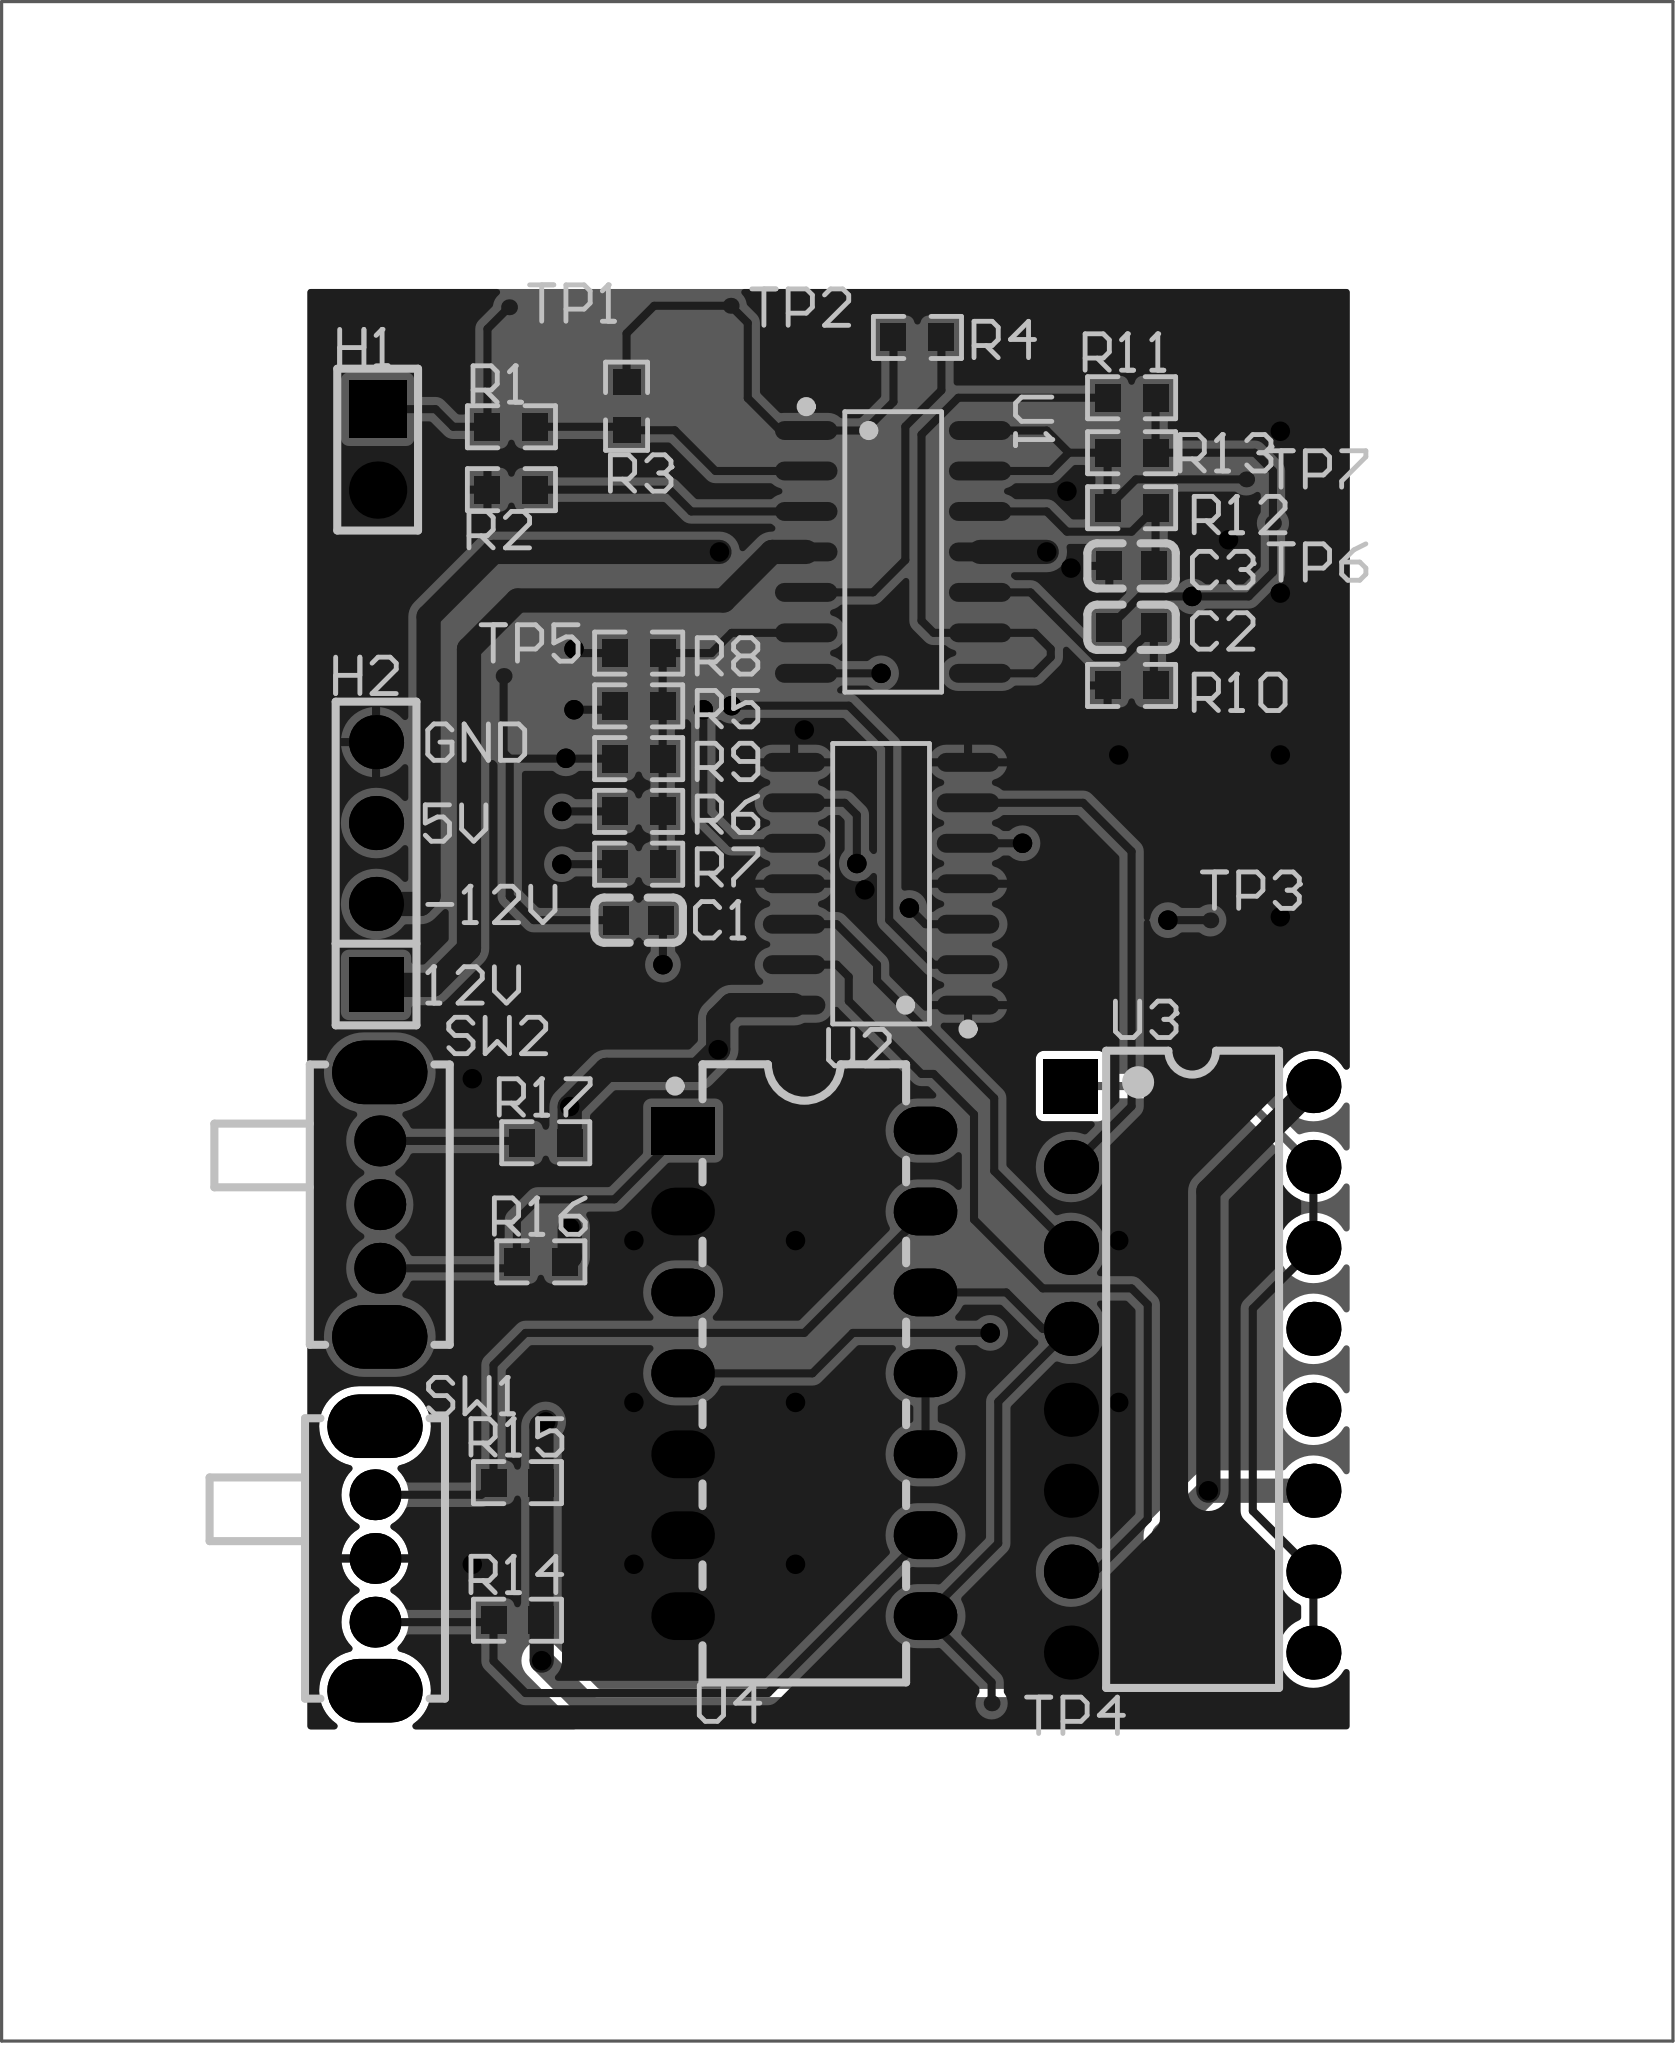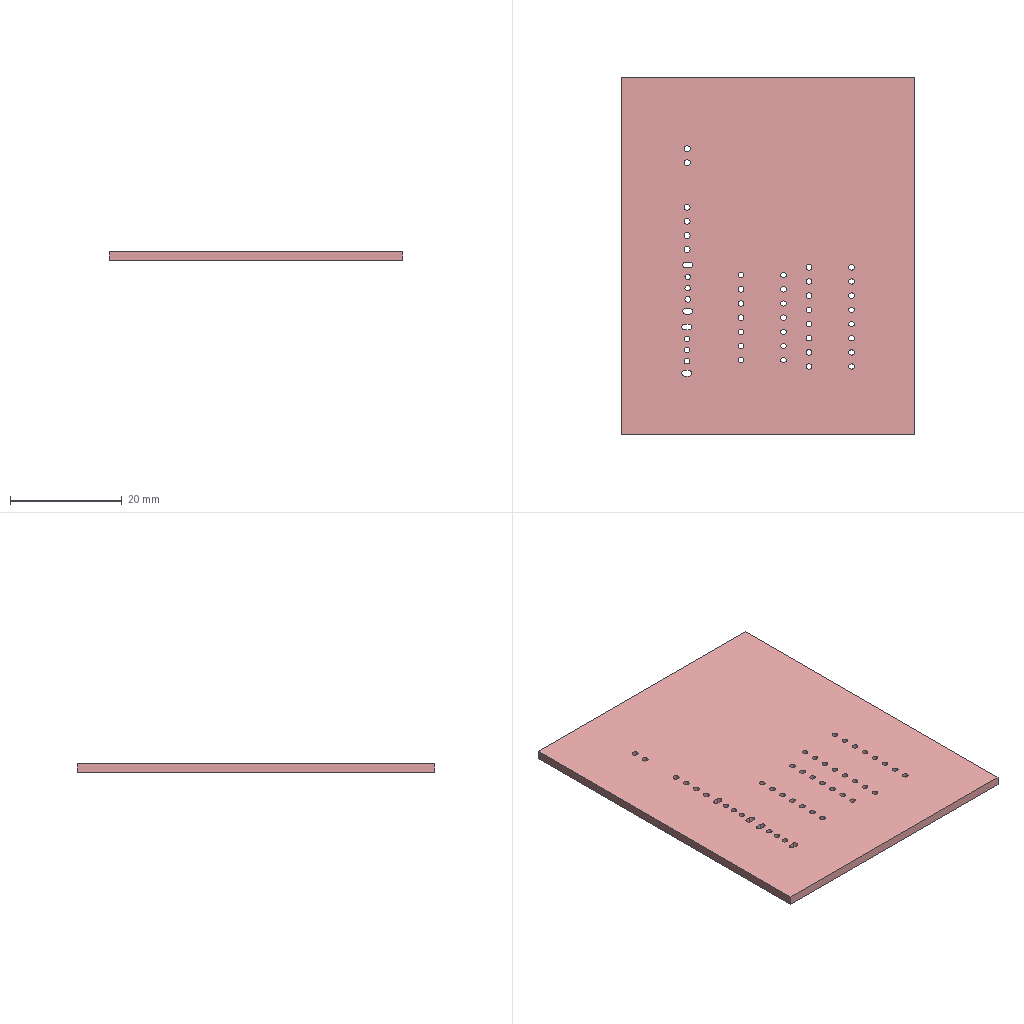Circuit board layout | Altium Designer | box 52.5 x 64 x 1.6 mm
Layer stack:
# Altium Designer layer stack of  (unit mm; dielectric type: 0 none, 1 core, 2 prepreg, 3 surface material)
index,name,kind,layer,copper_thickness_mm,dielectric_type,dielectric_thickness_mm,dielectric_material,dielectric_constant
0,Top Paste Mask Layer,other,,,,,,
1,Top Silkscreen Layer,other,,,,,,
2,Top Solder Mask Layer,dielectric,,,3,0.01,,3.3
3,Top Layer,copper,Top Layer,0.035,,,,
4,Dielectric1,dielectric,,,3,1.51,FR4,4.5
5,Bottom Layer,copper,Bottom Layer,0.035,,,,
6,Bottom Solder Mask Layer,dielectric,,,3,0.01,,3.3
7,Bottom Silkscreen Layer,other,,,,,,
8,Bottom Paste Mask Layer,other,,,,,,
# drill layer pairs: low layer,high layer
drill_pair,Top Layer,Bottom Layer
Part placement:
Designator,Comment,Layer,Footprint,Center-X(mm),Center-Y(mm),Rotation
C1,150nF,TopLayer,C0603,89.875,105.029,0
C2,150nF,TopLayer,C0603,105.369,114.221,0
C3,20nF,TopLayer,C0603,105.369,116.147,0
H1,,TopLayer,HDR-TH_2P-P2.54-V-M-1,81.67,119.796,270
H2,,TopLayer,HDR-TH_4P-P2.54-V-M,81.62,106.807,90
R3,1.2M,TopLayer,R0603,89.494,121.158,90
R4,10K,TopLayer,R0603,98.638,123.317,0
R5,80K,TopLayer,R0603,89.875,111.755,0
R6,40K,TopLayer,R0603,89.875,108.442,0
R7,20K,TopLayer,R0603,89.875,106.786,0
R8,10K,TopLayer,R0603,89.875,113.411,0
R9,160K,TopLayer,R0603,89.875,110.098,0
R10,15K,TopLayer,R0603,105.369,112.395,0
R11,15K,TopLayer,R0603,105.369,121.425,0
R12,1.5K,TopLayer,R0603,105.369,117.973,0
R13,1.5K,TopLayer,R0603,105.369,119.699,180
R14,1K,TopLayer,R0603,86.065,83.058,0
R15,1K,TopLayer,R0603,86.065,87.376,0
R16,1K,TopLayer,R0603,86.8,94.305,0
R17,1K,TopLayer,R0603,86.954,98.044,0
SW1,,TopLayer,拨动开关_侧,81.587,84.996,270
SW2,,TopLayer,拨动开关_侧,81.737,96.101,270
TP1,,TopLayer,Test-Point-0.5mm,85.801,124.264,0
TP2,,TopLayer,Test-Point-0.5mm,92.767,124.311,0
TP3,,TopLayer,Test-Point-0.5mm,107.844,105.022,0
TP4,,TopLayer,Test-Point-0.5mm,100.97,80.45,0
TP5,,TopLayer,Test-Point-0.5mm,85.63,112.691,0
TP6,,TopLayer,Test-Point-0.5mm,109.813,117.488,0
TP7,,TopLayer,Test-Point-0.5mm,108.972,118.862,0
U1,LM324ADR,TopLayer,SOP-14_L8.6-W3.9-P1.27-LS6.0-BL,97.876,116.586,270
U2,CD4066BD,TopLayer,SOP-14_L8.6-W3.9-P1.27-LS6.0-BL,97.495,106.172,90
U3,NTE74193,TopLayer,PDIP-16_L19.7-W6.6-P2.54-LS7.6-BL,107.274,90.932,270
U4,SN7400N,TopLayer,PDIP-14_L19.3-W6.4-P2.54-LS7.9-BL-1,95.082,90.805,270
R1,120K,TopLayer,R0603,85.876,120.513,0
R2,110K,TopLayer,R0603,85.876,118.54,0
Pad and via stacks:
# Altium Designer via and pad stacks of  (unit mm). Each distinct definition once, with the count of objects using it.
# via: kind,start_layer,end_layer,hole_mm,diameter_mm,mode(0 simple;1 top-mid-bottom;2 full stack),diameter_per_layer,count,example_net
# pad: kind,layer,hole_mm,hole_type(0 round;1 square;2 slot),plating,top_size,top_shape(1 round;2 rect;3 octagon;9 rounded rect),mid_size,bottom_size,mode,footprint,size_per_layer,count,example
pad,Top Layer,0,0,plated,0.8x0.9,2,0.8x0.9,0.8x0.9,0,C0603,,6,C1.2
pad,Top Layer,0,0,plated,0.8065x0.864,2,0.8065x0.864,0.8065x0.864,0,R0603,,34,R3.2
pad,Top Layer,0,0,plated,0.5x0.5,1,0.5x0.5,0.5x0.5,0,Test-Point-0.5mm,,7,TP1.1
pad,Top Layer,0,0,plated,0.595x1.968,1,0.595x1.968,0.595x1.968,0,SOP-14_L8.6-W3.9-P1.27-LS6.0-BL,,28,U1.1
pad,Multi-Layer,1.1,0,plated,1.8x1.8,1,1.8x1.8,1.8x1.8,0,HDR-TH_2P-P2.54-V-M-1,,1,H1.2
pad,Multi-Layer,1.1,0,plated,1.8x1.8,2,1.8x1.8,1.8x1.8,0,HDR-TH_2P-P2.54-V-M-1,,1,H1.1
pad,Multi-Layer,1.1,0,plated,1.7x1.7,2,1.7x1.7,1.7x1.7,0,HDR-TH_4P-P2.54-V-M,,1,H2.1
pad,Multi-Layer,1.1,0,plated,1.7x1.7,1,1.7x1.7,1.7x1.7,0,HDR-TH_4P-P2.54-V-M,,3,H2.2
pad,Multi-Layer,1.001,0,plated,1.6x1.6,1,1.6x1.6,1.6x1.6,0,\u00B2\u00A6\u00B6\u00AF\u00BF\u00AA\u00B9\u00D8_\u00B2\u00E0,,6,SW1.1
pad,Multi-Layer,1.001,2,plated,3x1.999,1,3x1.999,3x1.999,0,\u00B2\u00A6\u00B6\u00AF\u00BF\u00AA\u00B9\u00D8_\u00B2\u00E0,,4,SW1.4
pad,Multi-Layer,1,0,plated,1.7x1.7,2,1.7x1.7,1.7x1.7,0,PDIP-16_L19.7-W6.6-P2.54-LS7.6-BL,,1,U3.1
pad,Multi-Layer,1,0,plated,1.7x1.7,1,1.7x1.7,1.7x1.7,0,PDIP-16_L19.7-W6.6-P2.54-LS7.6-BL,,15,U3.2
pad,Multi-Layer,1,0,plated,2x1.5,2,2x1.5,2x1.5,0,PDIP-14_L19.3-W6.4-P2.54-LS7.9-BL-1,,1,U4.1
pad,Multi-Layer,1,0,plated,2x1.5,1,2x1.5,2x1.5,0,PDIP-14_L19.3-W6.4-P2.54-LS7.9-BL-1,,13,U4.2
via,Top Layer,Bottom Layer,0.3048,0.61,0,,43,$1N23
Copper pours:
name,layer,net,type(0 solid;1 hatched;2 none)
Top Layer-GND,Top Layer,GND,0
Bottom Layer-GND,Bottom Layer,GND,0